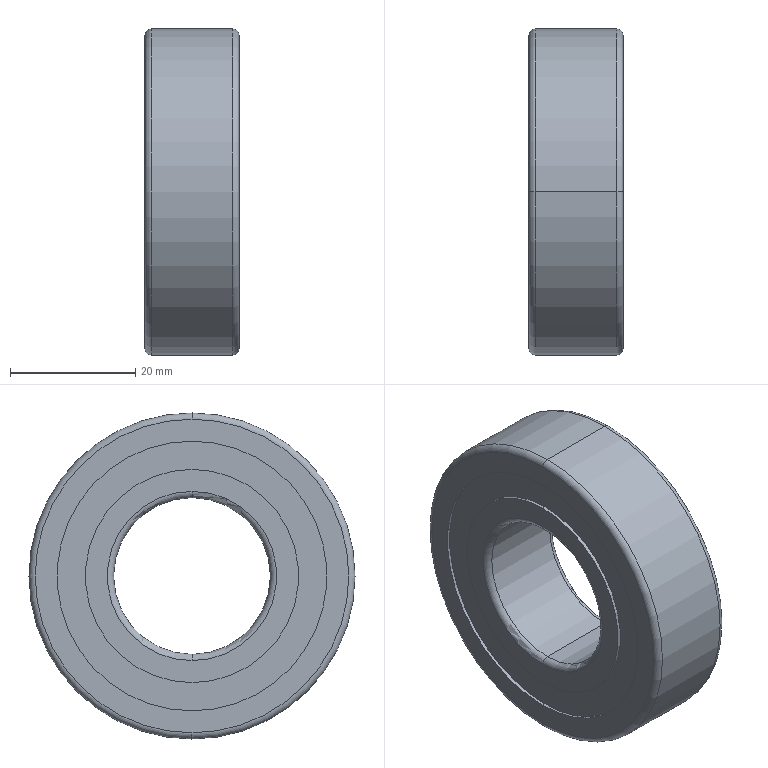Part | SolidWorks | features Revolution 3, CirPattern 1, RefAxis 1 | 18 solids | 90 faces | box 15 x 52 x 52 mm | volume 18682 mm3 | sphere 30 | cylinder 24 | torus 14 | cone 12 | plane 10 | commonest cylinder face diameters 34 x6 43 x6 32 x4 45 x4 25 x2 52 x2